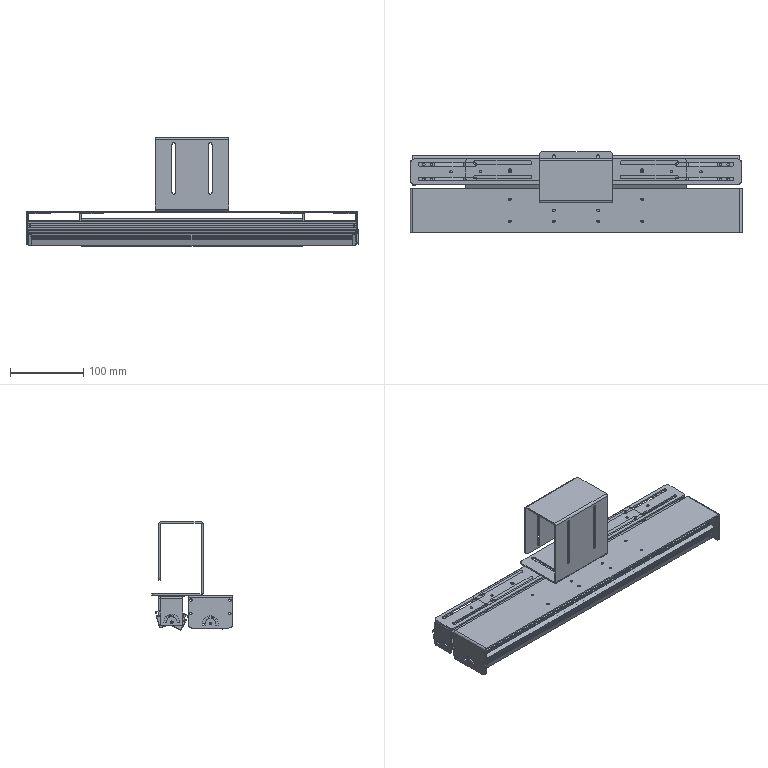Part | SolidWorks | 65 solids | 8313 faces | volume 517771 mm3 | spline 2880 | cylinder 2384 | plane 2369 | cone 680 | commonest cylinder face diameters 2 x1158 1.9 x576 0.2 x246 3.3 x108 0.6 x72 4 x56